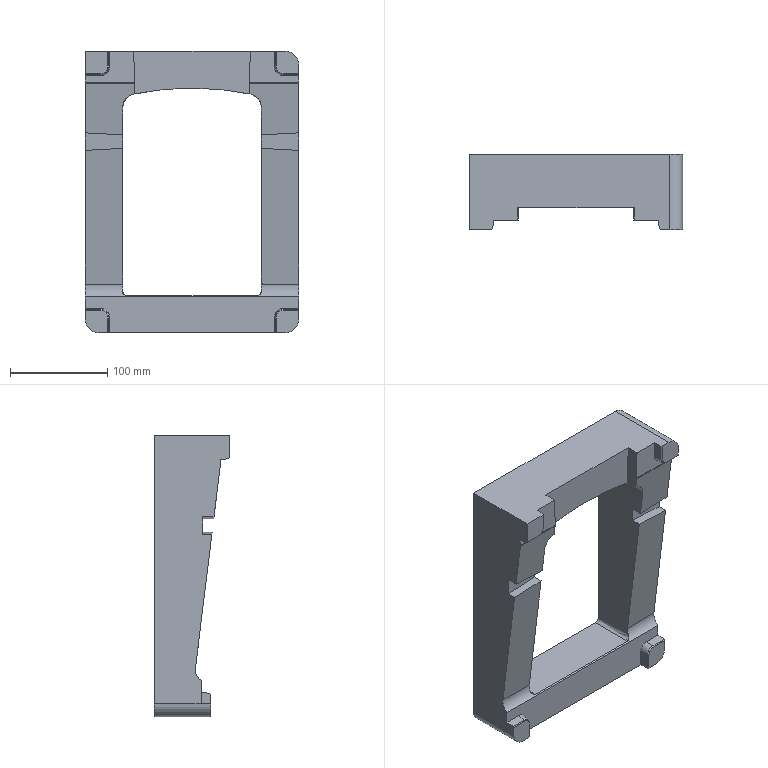Part | STEP file | 1 solid | 90 faces | box 220 x 78 x 290 mm | volume 1840139 mm3 | plane 55 | spline 23 | cylinder 12 | commonest cylinder face diameters 16 x4 27 x3 9.045 x2 20 x2 28.14 x1